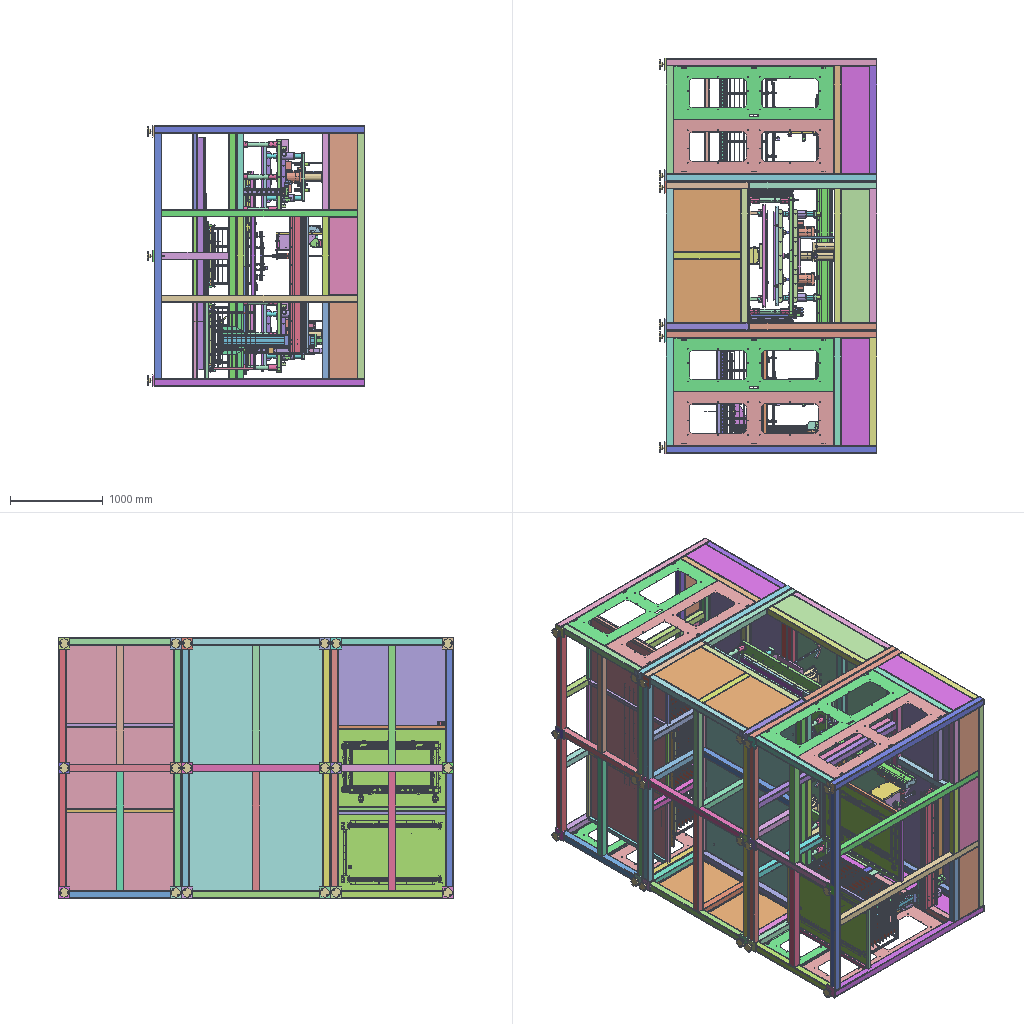Assembly | STEP file | 134 different items | 791 placed | box 2340 x 4246 x 2800 mm
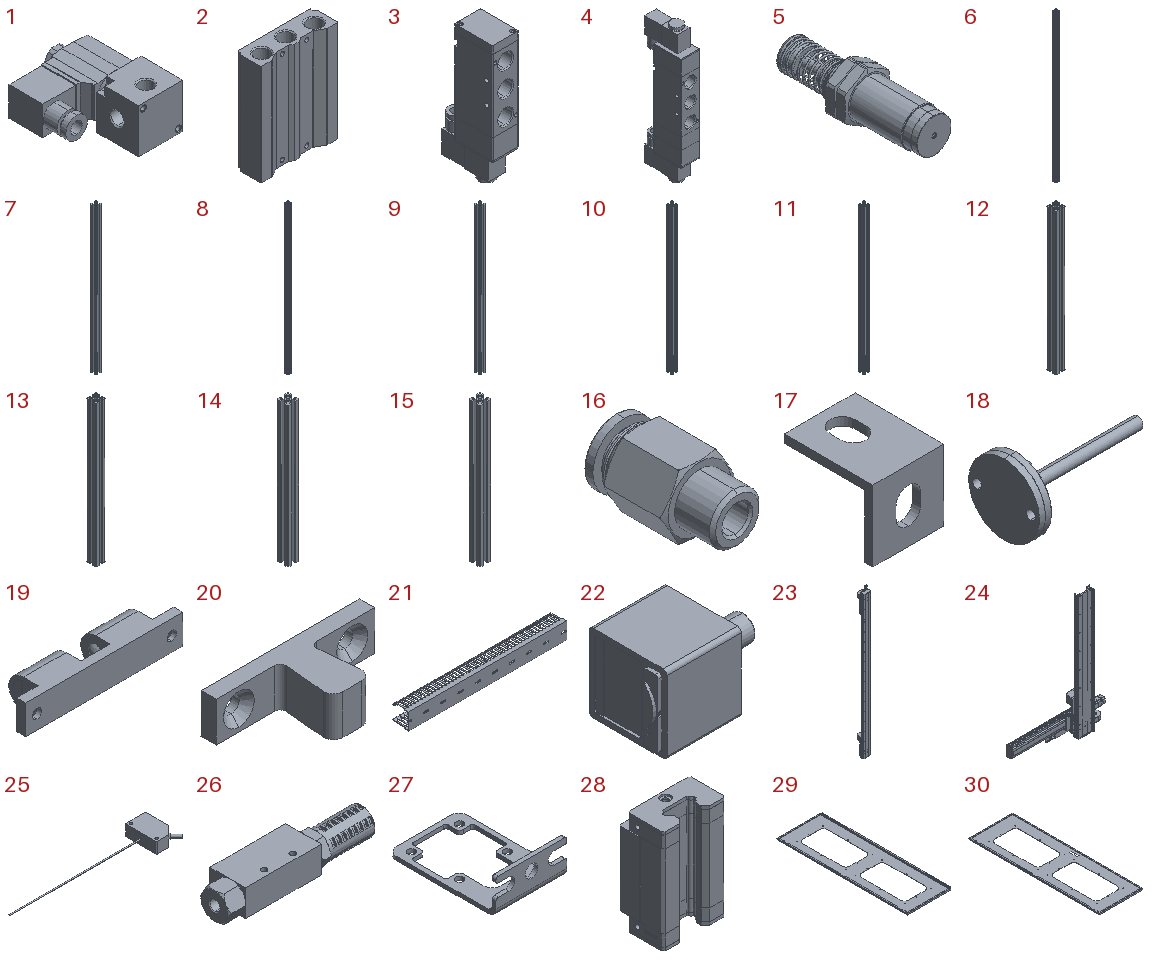Parts list (item | name | quantity | parent item | size | volume):
1 | 3V308NCB | x3 | in KF-2212-050-000, KF-2212-060-000 | 71.5 x 90.9 x 38 mm | 121350 mm3
2 | 400M3F | x2 | in Solenoid valve manifold | 100 x 33 x 131 mm | 261917 mm3
3 | 4V41015B | x2 | in Solenoid valve manifold | - | -
4 | 4V430E15B | x4 | in Solenoid valve manifold | 34 x 74.3 x 243.8 mm | 351634 mm3
5 | ACJ4225F-AirTAC | x8 | in TJ-DHQM-003-000 | 50 x 161.5 x 56.022 mm | 187281 mm3
6 | AOB02-H2020_YHD010 | x3 | in KF-2212-050-000, KF-2212-060-000 | 20 x 20 x 842 mm | 145364 mm3
7 | AOB02-H2020_YHD011 | x3 | in KF-2212-050-000, KF-2212-060-000 | 20 x 20 x 520 mm | 89774 mm3
8 | AOB02-H2020_YHD012 | x3 | in KF-2212-050-000, KF-2212-060-000 | 20 x 20 x 842 mm | 145364 mm3
9 | AOB02-H2020_YHD013 | x3 | in KF-2212-050-000, KF-2212-060-000 | 20 x 20 x 520 mm | 89774 mm3
10 | AOB02-H2020_YHD014 | x3 | in KF-2212-050-000, KF-2212-060-000 | 20 x 20 x 480 mm | 82868 mm3
11 | AOB02-H2020_YHD015 | x3 | in KF-2212-050-000, KF-2212-060-000 | 20 x 20 x 480 mm | 82868 mm3
12 | AOB02-H2020_YHD016 | x3 | in KF-2212-050-000, KF-2212-060-000 | 20 x 20 x 300 mm | 51792 mm3
13 | AOB02-H2020_YHD017 | x3 | in KF-2212-050-000, KF-2212-060-000 | 20 x 20 x 300 mm | 51792 mm3
14 | AOB02-H2020_YHD018 | x3 | in KF-2212-050-000, KF-2212-060-000 | 20 x 20 x 251 mm | 43333 mm3
15 | AOB02-H2020_YHD019 | x3 | in KF-2212-050-000, KF-2212-060-000 | 20 x 20 x 251 mm | 43333 mm3
16 | BPC1002 | x8 | in TJ-DHQM-003-000 | 19.63 x 32 x 17 mm | 3663 mm3
17 | BRACKET_0829_041_CRONWB29 | x12 | in 0829_041_CRONWB29 | 20 x 25 x 20 mm | 1691 mm3
18 | C-CPVCH16-150 | x18 | in Frame | 190 x 100 x 100 mm | 196270 mm3
19 | CATCHE1_MISUMI_BCAS70_Latch | x6 | in MISUMI_BCAS70_Latch | 70 x 17 x 13 mm | 9236 mm3
20 | CATCHE2_MISUMI_BCAS70_Latch | x6 | in MISUMI_BCAS70_Latch | 42 x 19 x 10.5 mm | 2994 mm3
21 | Cable tray1_1495 | x4 | in TJ-DHQM-003-000 | 460 x 47.5 x 48 mm | 74252 mm3
22 | DPSN101020 | x3 | in KF-2212-050-000, KF-2212-060-000 | 46.1 x 30 x 30 mm | 26185 mm3
23 | EH17B-L13-C-S3000-ZP75-D3-N10 | x1 | in KF-2212-050-000 | - | 18933367 mm3
24 | EH17BEH13-F-3000-600+150BC-W221226YJ01 | x1 | in KF-2212-060-000 | 1159 x 261.907 x 1561 mm | 18211438 mm3
25 | ES201-R10MN (Huayifeng) | x3 | in KF-2212-070-000 | 154.334 x 37.365 x 10.8 mm | 6448 mm3
26 | EV-20 | x3 | in KF-2212-050-000, KF-2212-060-000 | 165.5 x 42.263 x 30 mm | 136290 mm3
27 | F-DPSLB | x3 | in KF-2212-050-000, KF-2212-060-000 | 29.6 x 45 x 14.7 mm | 1443 mm3
28 | HGH35C | x6 | in TJ-DHQM-004-000 | 70 x 47.5 x 112.4 mm | 276753 mm3
29 | Hinged door 1-left | x4 | in Assembly 1^Frame | 587.5 x 1721 x 21.7 mm | 1104799 mm3
30 | Hinged door 1-right | x4 | in Assembly 1^Frame | 574 x 1721 x 20 mm | 1096679 mm3
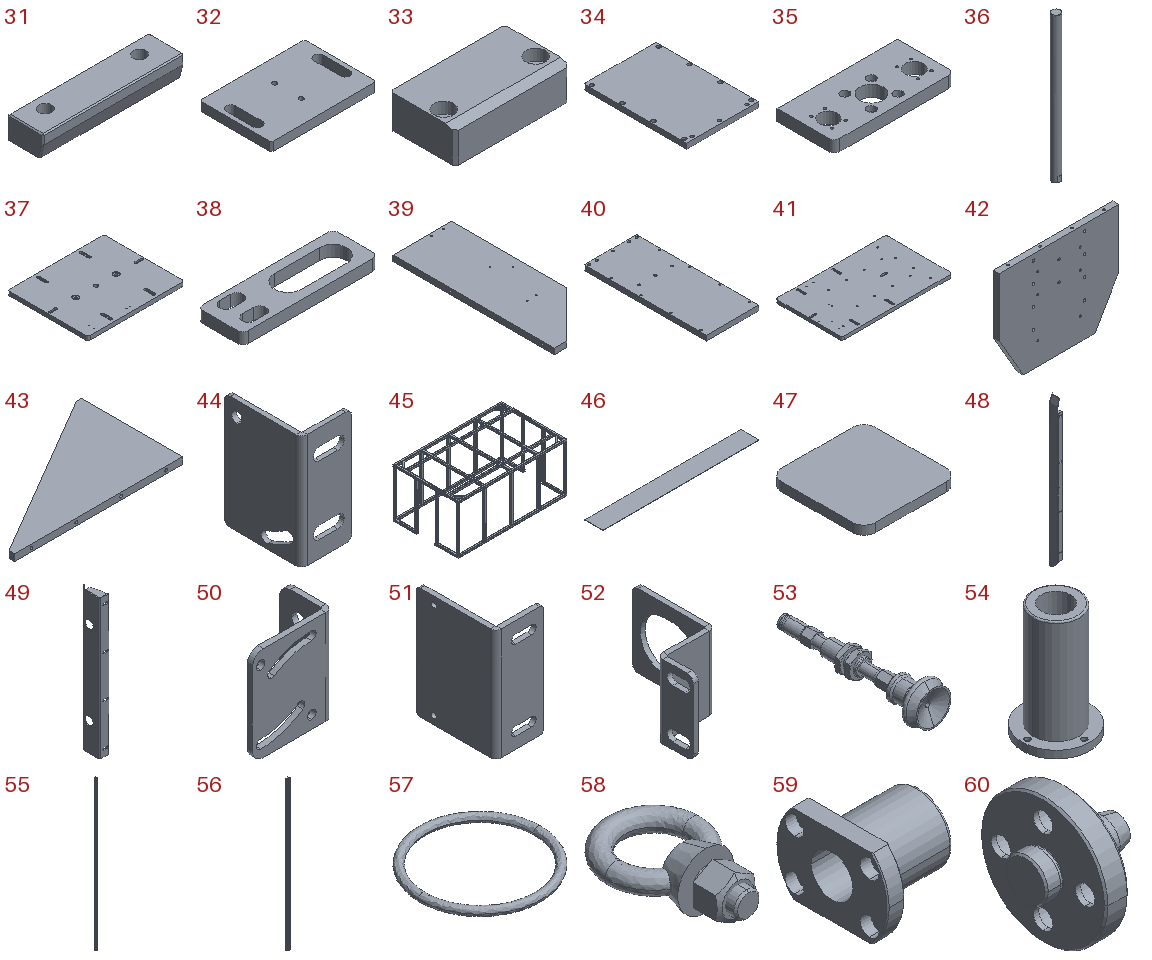31 | KF-2212-010-049 | x4 | in KF-2212-010-1 | 60 x 15 x 10 mm | 7567 mm3
32 | KF-2212-010-050 | x4 | in KF-2212-010-1 | 60 x 41 x 5 mm | 11178 mm3
33 | KF-2212-010-051 | x4 | in KF-2212-010-1 | 35 x 20 x 10 mm | 6626 mm3
34 | KF-2212-050-001 | x2 | in KF-2212-050-000 | 210 x 300 x 15 mm | 931509 mm3
35 | KF-2212-050-002 | x2 | in KF-2212-050-000 | 210 x 100 x 20 mm | 347402 mm3
36 | KF-2212-050-003 | x4 | in KF-2212-050-000 | 20 x 20 x 350 mm | 109026 mm3
37 | KF-2212-050-004 | x2 | in KF-2212-050-000 | 360 x 300 x 15 mm | 1590631 mm3
38 | KF-2212-050-005 | x36 | in KF-2212-050-000, KF-2212-060-000 | 60 x 20 x 5 mm | 3695 mm3
39 | KF-2212-050-006 | x4 | in KF-2212-050-000 | 153 x 420 x 15 mm | 852381 mm3
40 | KF-2212-050-007 | x2 | in KF-2212-050-000 | 210 x 490 x 20 mm | 2037060 mm3
41 | KF-2212-060-001 | x1 | in KF-2212-060-000 | 500 x 300 x 15 mm | 2214931 mm3
42 | KF-2212-060-002 | x1 | in KF-2212-060-000 | 300 x 15 x 250 mm | 1020222 mm3
43 | KF-2212-060-003 | x2 | in KF-2212-060-000 | 300 x 180 x 12 mm | 349451 mm3
44 | KF-2212-060-004 | x1 | in KF-2212-060-000 | 22 x 34 x 50 mm | 4893 mm3
45 | KF-2212-070-001_Default<As Machined> | x3 | in KF-2212-070-000 | 1036 x 620 x 470 mm | 2149735 mm3
46 | KF-2212-070-002 | x6 | in KF-2212-070-000 | 1036 x 120 x 2 mm | 248629 mm3
47 | KF-2212-070-003 | x12 | in KF-2212-070-000 | 16 x 16 x 1.5 mm | 378.85 mm3
48 | KF-2212-070-004 | x3 | in KF-2212-070-000 | 30 x 71.142 x 1037 mm | 309462 mm3
49 | KF-2212-070-005 | x3 | in KF-2212-070-000 | 33 x 74.142 x 500 mm | 165565 mm3
50 | KF-2212-070-006 | x3 | in KF-2212-070-000 | 30 x 18 x 35 mm | 2796 mm3
51 | KF-2212-070-007 | x6 | in KF-2212-070-000 | 30 x 50 x 70 mm | 17137 mm3
52 | KF-2212-070-008 | x3 | in KF-2212-070-000 | 22 x 45 x 30 mm | 2910 mm3
53 | KF-MISUMI_C-MPTBN-B20 suction cup | x36 | in KF-2212-050-000, KF-2212-060-000 | 25 x 95.1 x 25 mm | 9058 mm3
54 | LMG02-d50-Yiheda | x8 | in TJ-DHQM-003-000 | 116 x 116 x 192 mm | 653566 mm3
55 | Linear rail HG25 (HIWIN) | x2 | in Frame | 23 x 22 x 2500 mm | 1042897 mm3
56 | Linear rail HG35  L2120 (HIWIN) | x2 | in TJ-DHQM-004-000 | 34 x 29 x 2120 mm | 1725609 mm3
57 | M-ORP40-3 | x4 | in TJ-DHQM-004-000 | 46 x 46 x 3 mm | 954.884 mm3
58 | M16-Lifting eye | x8 | in TJ-DHQM-003-000 | 61.5 x 90.6 x 35.3 mm | 37230 mm3
59 | MISUMI_LHFCM20_Linear Bearing-2 | x4 | in KF-2212-050-000 | 42 x 54 x 38 mm | 27416 mm3
60 | MISUMI_MASAA12-P10.00-B10.0-T7.0_Locating pin | x1 | in TJ-DHQM-004-000 | 26 x 36 x 36 mm | 6932 mm3
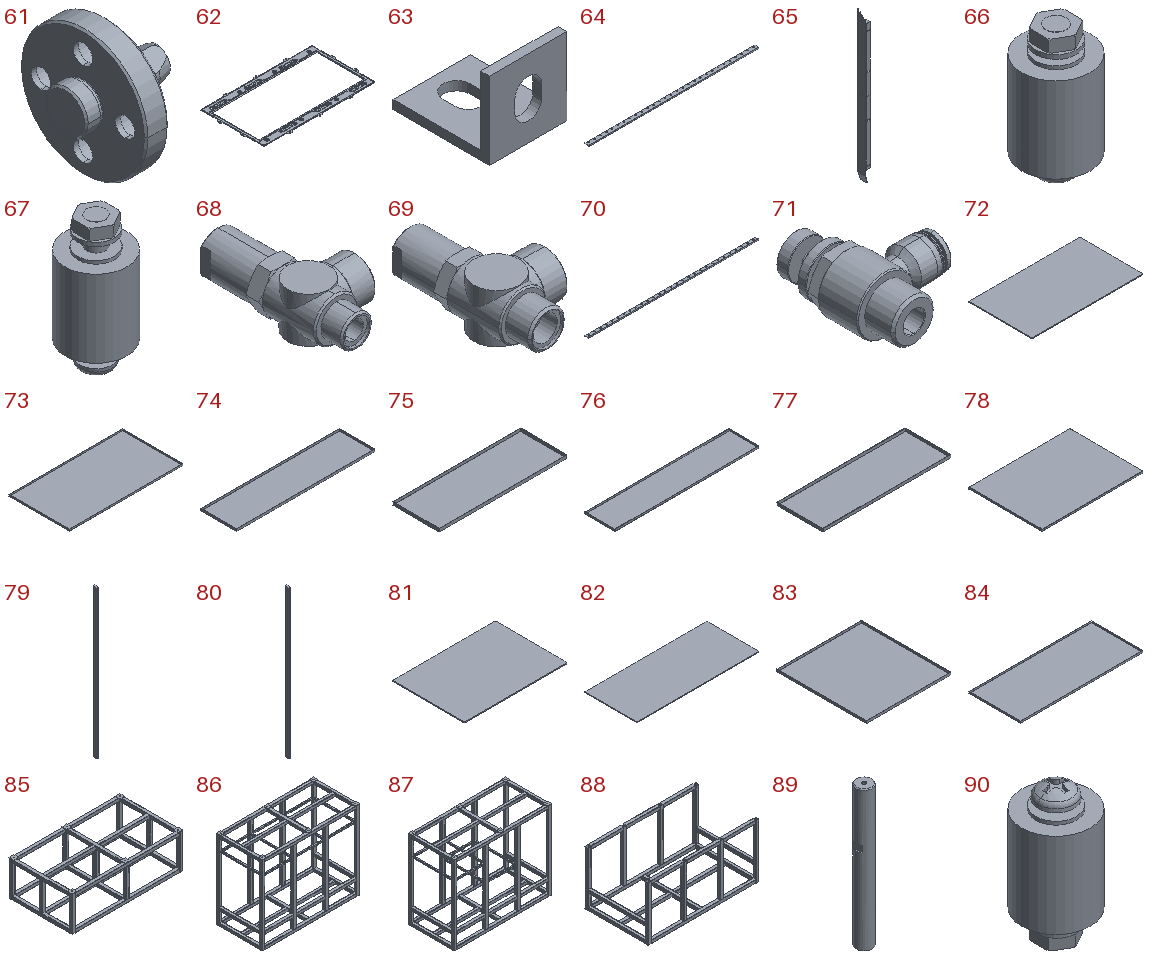61 | MISUMI_MASDA12-P10.00-B10.0-T7.0_Locating pin | x1 | in TJ-DHQM-004-000 | 26 x 36 x 36 mm | 6690 mm3
62 | Membrane frame | x35 | in General assembly, KF-2212-010-1, KF-2212-050-000, KF-2212-060-000, KF-2212-070-000 | 988 x 574 x 3 mm | 383465 mm3
63 | Mirror BRACKET_0829_041_CRONWB29 | x12 | in Mirror 0829_041_CRONWB29 | 20 x 25 x 20 mm | 1691 mm3
64 | Mirror PLATE_0829_041_CRONWB29 | x6 | in Mirror 0829_041_CRONWB29 | 1013 x 25 x 7 mm | 47472 mm3
65 | Mirror Part 3 | x3 | in KF-2212-070-000 | 30 x 71.142 x 1037 mm | 319137 mm3
66 | Mirror ROLLER-1_0829_041_CRONWB29 | x81 | in Mirror 0829_041_CRONWB29 | 20 x 20 x 38.858 mm | 8836 mm3
67 | Mirror ROLLER-2_0829_041_CRONWB29 | x6 | in Mirror 0829_041_CRONWB29 | 20 x 20 x 43.458 mm | 8966 mm3
68 | PCV10 | x4 | in TJ-DHQM-003-000 | 37.702 x 74.5 x 24 mm | 30380 mm3
69 | PCV15 | x8 | in TJ-DHQM-003-000 | 41.856 x 79.5 x 28 mm | 41783 mm3
70 | PLATE_0829_041_CRONWB29 | x6 | in 0829_041_CRONWB29 | 1013 x 25 x 7 mm | 47472 mm3
71 | PSL1004A | x8 | in TJ-DHQM-003-000 | 49.5 x 58.5 x 28 mm | 24100 mm3
72 | Part 1 | x1 | in Frame | 2800 x 1600 x 20 mm | 89598283 mm3
73 | Part 10 | x4 | in Frame | 1280 x 680 x 20 mm | 1876066 mm3
74 | Part 11 | x4 | in Frame | 1160 x 300 x 20 mm | 796554 mm3
75 | Part 12 | x4 | in Frame | 820 x 300 x 20 mm | 568950 mm3
76 | Part 13 | x2 | in Frame | 1440 x 300 x 20 mm | 983993 mm3
77 | Part 14 | x2 | in Frame | 840 x 300 x 20 mm | 582338 mm3
78 | Part 15 | x2 | in Frame | 1160 x 840 x 20 mm | 2086843 mm3
79 | Part 16 | x1 | in Frame | 25 x 62 x 2500 mm | 3760000 mm3
80 | Part 17 | x1 | in Frame | 25 x 60 x 2500 mm | 3750000 mm3
81 | Part 2 | x1 | in Frame | 1600 x 1120 x 15 mm | 26878712 mm3
82 | Part 6 | x1 | in Frame | 2720 x 1160 x 15 mm | 47326712 mm3
83 | Part 8 | x4 | in Frame | 680 x 720 x 20 mm | 1075588 mm3
84 | Part 9 | x8 | in Frame | 1280 x 540 x 20 mm | 1507947 mm3
85 | Part3_default<as machined> | x1 | in Frame | 2800 x 1600 x 895 mm | 31350509 mm3
86 | Part4_default<as machined> | x1 | in Frame | 2800 x 1320 x 2280 mm | 47206904 mm3
87 | Part5_default<as machined> | x1 | in Frame | 2800 x 1320 x 2280 mm | 46678246 mm3
88 | Part7_default<as machined> | x1 | in Frame | 2800 x 1600 x 1380 mm | 29274094 mm3
89 | RAD36-D50-L435-SC150-M12-N12-Yiheda | x12 | in TJ-DHQM-003-000 | 50 x 50 x 435 mm | 845554 mm3
90 | ROLLER-1_0829_041_CRONWB29 | x81 | in 0829_041_CRONWB29 | 20 x 20 x 38.858 mm | 8836 mm3
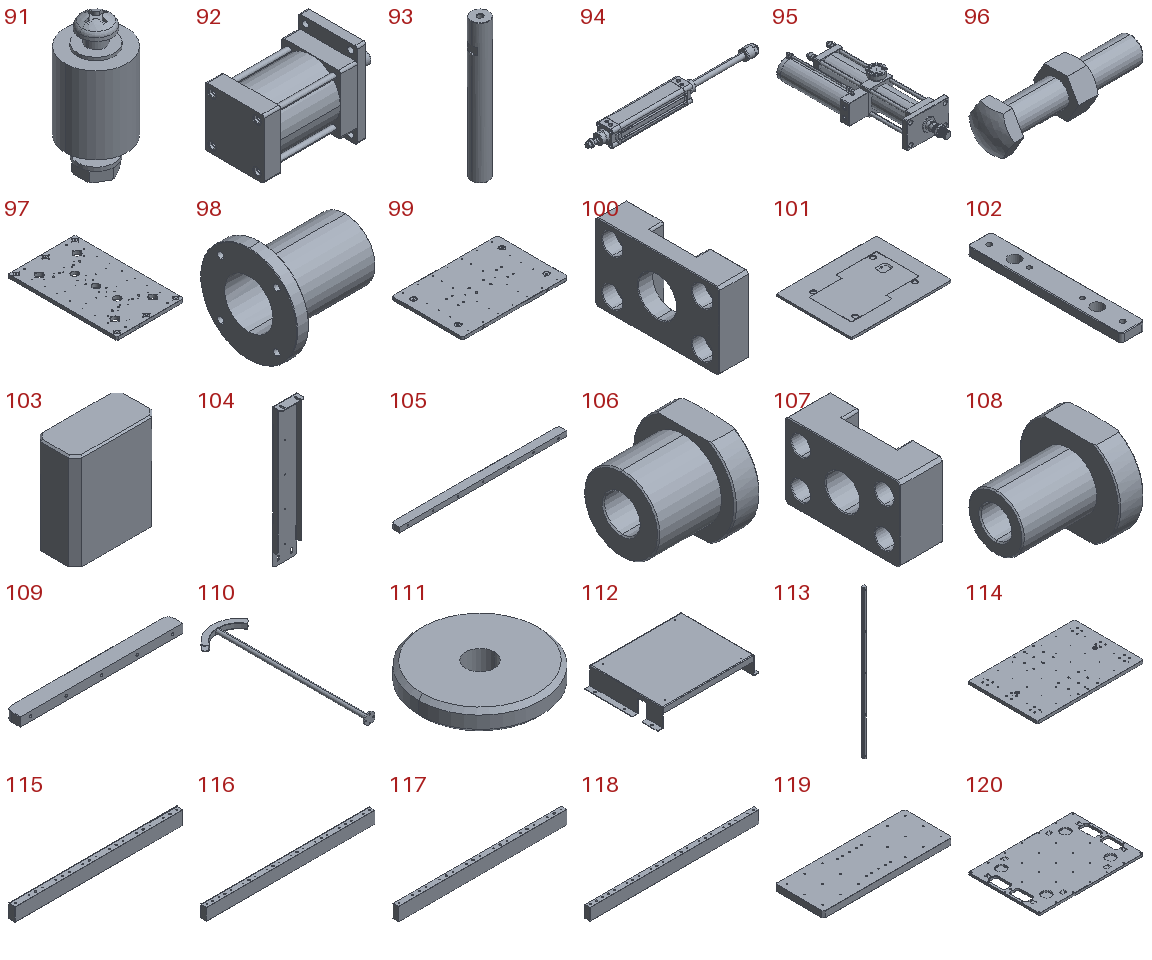91 | ROLLER-2_0829_041_CRONWB29 | x6 | in 0829_041_CRONWB29 | 20 x 20 x 43.458 mm | 8966 mm3
92 | SC125X100SFA_000_ | x4 | in TJ-DHQM-003-000 | 303 x 136 x 196 mm | 2823213 mm3
93 | SCK02-D50-L390-M16-N16-S60-Yiheda | x8 | in TJ-DHQM-003-000 | 50 x 50 x 390 mm | 752032 mm3
94 | SEJ50x200-20S_0020_+_DMSE-2_ | x2 | in KF-2212-050-000 | 651 x 64.6 x 64 mm | 961135 mm3
95 | STA-80-100-10-5T-Xuntuo | x2 | in TJ-DHQM-003-000 | 240 x 641 x 158.4 mm | 3516395 mm3
96 | STBB16-80-MISIMI | x8 | in TJ-DHQM-003-000 | 90 x 27.7 x 24 mm | 24665 mm3
97 | TJ-DHQM-003-001 | x2 | in TJ-DHQM-003-000 | 800 x 1300 x 40 mm | 39783539 mm3
98 | TJ-DHQM-003-002_STHRBK30 | x24 | in TJ-DHQM-003-000 | 100 x 100 x 100 mm | 160939 mm3
99 | TJ-DHQM-003-003 | x2 | in TJ-DHQM-003-000 | 1070 x 720 x 30 mm | 22699687 mm3
100 | TJ-DHQM-003-004 | x2 | in TJ-DHQM-003-000 | 48 x 200 x 124 mm | 792804 mm3
101 | TJ-DHQM-003-005 | x2 | in TJ-DHQM-003-000 | 950 x 720 x 20 mm | 13492361 mm3
102 | TJ-DHQM-003-006 | x4 | in TJ-DHQM-003-000 | 80 x 520 x 30 mm | 1140560 mm3
103 | TJ-DHQM-003-007 | x8 | in TJ-DHQM-003-000 | 100 x 50 x 115 mm | 555425 mm3
104 | TJ-DHQM-003-008 | x4 | in TJ-DHQM-003-000 | 80 x 30 x 465 mm | 103088 mm3
105 | TJ-DHQM-003-009 | x8 | in TJ-DHQM-003-000 | 1000 x 50 x 30 mm | 1451710 mm3
106 | TJ-DHQM-003-010 | x2 | in TJ-DHQM-003-000 | 73 x 82 x 70 mm | 202408 mm3
107 | TJ-DHQM-003-011 | x4 | in TJ-DHQM-003-000 | 60 x 160 x 104 mm | 672141 mm3
108 | TJ-DHQM-003-012 | x4 | in TJ-DHQM-003-000 | 83 x 82 x 70 mm | 162318 mm3
109 | TJ-DHQM-003-013 | x16 | in TJ-DHQM-003-000 | 550 x 50 x 30 mm | 789176 mm3
110 | TJ-DHQM-003-014 | x2 | in TJ-DHQM-003-000 | 208.431 x 730 x 50 mm | 102076 mm3
111 | TJ-DHQM-003-015 | x8 | in TJ-DHQM-003-000 | 30 x 30 x 5 mm | 3250 mm3
112 | TJ-DHQM-003-016 | x2 | in TJ-DHQM-003-000 | 446 x 320 x 80 mm | 405095 mm3
113 | TJ-DHQM-003-017 | x4 | in TJ-DHQM-003-000 | 15 x 13 x 720 mm | 103094 mm3
114 | TJ-DHQM-004-001 | x2 | in TJ-DHQM-004-000 | 1100 x 720 x 30 mm | 23583898 mm3
115 | TJ-DHQM-004-002 | x1 | in TJ-DHQM-004-000 | 1000 x 37.5 x 82.5 mm | 2965048 mm3
116 | TJ-DHQM-004-003 | x1 | in TJ-DHQM-004-000 | 1120 x 37.5 x 82.5 mm | 3313351 mm3
117 | TJ-DHQM-004-004 | x1 | in TJ-DHQM-004-000 | 1000 x 35 x 80 mm | 2758827 mm3
118 | TJ-DHQM-004-005 | x1 | in TJ-DHQM-004-000 | 1120 x 35 x 80 mm | 3082362 mm3
119 | TJ-DHQM-004-006 | x2 | in TJ-DHQM-004-000 | 720 x 270 x 35 mm | 6743706 mm3
120 | TJ-DHQM-004-007 | x2 | in TJ-DHQM-004-000 | 920 x 630 x 20 mm | 10320412 mm3
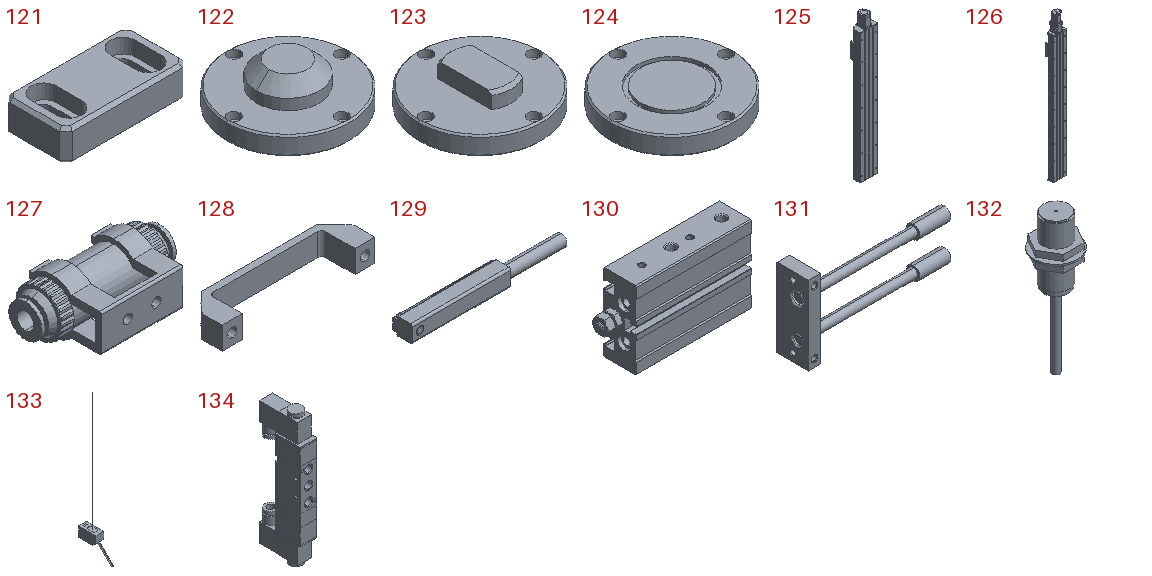121 | TJ-DHQM-004-008 | x8 | in TJ-DHQM-004-000 | 39 x 20 x 10 mm | 5997 mm3
122 | TJ-DHQM-004-009 | x2 | in TJ-DHQM-004-000 | 79.9 x 79.9 x 27 mm | 74312 mm3
123 | TJ-DHQM-004-010 | x2 | in TJ-DHQM-004-000 | 79.9 x 79.9 x 22 mm | 66197 mm3
124 | TJ-DHQM-004-011 | x4 | in TJ-DHQM-004-000 | 79.9 x 79.9 x 12 mm | 57718 mm3
125 | TPA-HNR-175D-2510C-L1000-M-C-P75-N3 | x1 | in Frame | 188.7 x 103 x 1435 mm | 7507272 mm3
126 | TPA-HNR-175D-2525C-L1400-M-C-J90-N3 | x1 | in TJ-DHQM-004-000 | - | -
127 | VFD-03-08 | x3 | in KF-2212-050-000, KF-2212-060-000 | 65.2 x 35.25 x 26 mm | 26161 mm3
128 | XAB57-L100 | x4 | in TJ-DHQM-003-000 | 115 x 30 x 17 mm | 14990 mm3
129 | _CMSG_GN | x8 | in TR6X10S_0_+_CMSG-2_ | 40.5 x 5.8 x 4.4 mm | 628.814 mm3
130 | _TR6-1010_b | x4 | in TR6X10S_0_+_CMSG-2_ | 63 x 16 x 37 mm | 25350 mm3
131 | _TR6-10_fr | x4 | in TR6X10S_0_+_CMSG-2_ | 65.5 x 14 x 35 mm | 4387 mm3
132 | gx-118m | x3 | in KF-2212-070-000 | 29 x 29 x 94 mm | 14418 mm3
133 | hg-c series | x1 | in KF-2212-060-000 | 20 x 76.982 x 357.882 mm | 21957 mm3
134 | 三位五通阀4V330C-08-Valve_Body | x2 | in KF-2212-050-000 | - | -